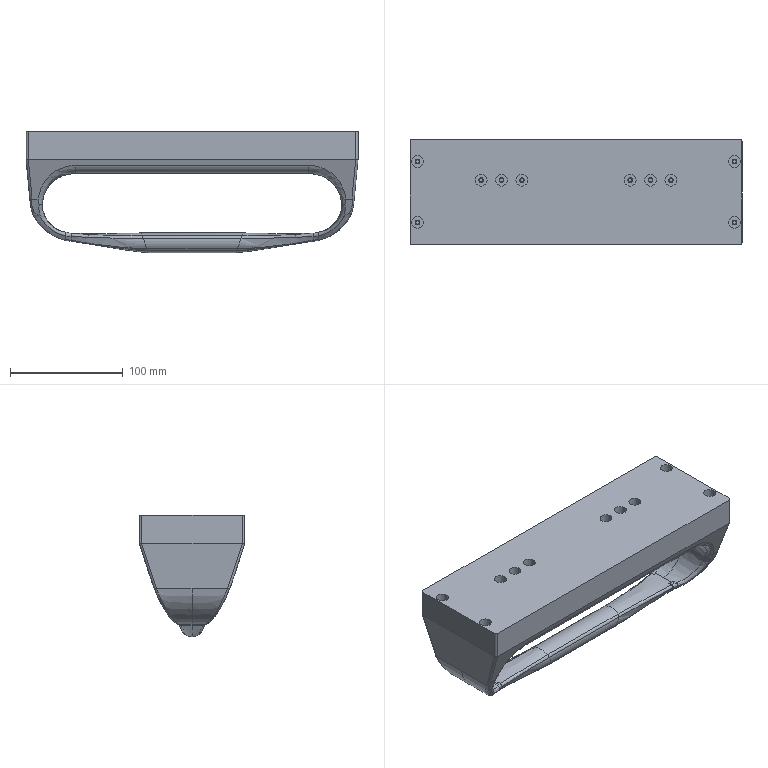NC program | NX | posted with a generic post | part box 294.078 x 93.5 x 107.5 mm
Lines 259 to 1268 of 185821:
(FIXED_CONTOUR , TOOL : D10R2)
N510 T09 M6
N512 G54
N514 G17 G0 G90 X46.702 Y-88.559 B0. C0. S7500 M3
N516 G43 Z30. H9
N518 Z-38.
N520 G94 G1 Z-40.107 F1000.
N522 X46.572 Y-88.43 Z-40.758
N524 X46.19 Y-88.155 Z-41.249
N526 X45.652 Y-87.879 Z-41.566
N528 X45.035 Y-87.652 Z-41.756
N530 X44.381 Y-87.48 Z-41.862
N532 X43.709 Y-87.358 Z-41.91
N534 X43.028 Y-87.278 Z-41.915
N536 X42.345 Y-87.233 Z-41.889
N538 X41.662 Y-87.22 Z-41.839
N540 X41.011 Z-41.785 F2500.
N542 X40.495 Z-41.758
N544 X39.805 Z-41.735
N546 X39.174 Z-41.73
N548 X20.152 Y-87.219
N550 X-39.177 Y-87.218 Z-41.726
N552 X-39.809 Z-41.732
N554 X-40.44 Z-41.755
N556 X-41.072 Z-41.793
N558 X-41.631 Z-41.84
N560 X-42.336 Y-87.186 Z-41.848
N562 X-42.568 Y-87.171 Z-41.851
N564 X-42.336 Z-41.821
N566 X-41.704 Z-41.756
N568 X-41.072 Z-41.705
N570 X-40.44 Z-41.669
N572 X-39.809 Z-41.648
N574 X-39.177 Z-41.642
N576 X17.515 Y-87.173 Z-41.646
N578 X32.819 Z-41.647
N580 X39.244 Z-41.646
N582 X39.805 Z-41.65
N584 X40.437 Z-41.67
N586 X41.069 Z-41.703
N588 X41.631 Z-41.748
N590 X41.701 Z-41.753
N592 X42.333 Z-41.817
N594 X42.596 Z-41.85
N596 X43.362 Y-87.127 Z-41.857
N598 X43.223 Z-41.836
N600 X42.965 Z-41.803
N602 X42.707 Z-41.775
N604 X42.333 Z-41.728
N606 X42.075 Z-41.704
N608 X41.701 Z-41.666
N610 X41.443 Z-41.651
N612 X41.069 Z-41.62
N614 X40.437 Z-41.587
N616 X40.179 Z-41.582
N618 X39.805 Z-41.57
N620 X39.174 Y-87.126 Z-41.566
N622 X15.94 Z-41.565
N624 X-39.177 Y-87.125 Z-41.562
N626 X-39.809 Z-41.567
N628 X-40.44 Z-41.587
N630 X-41.072 Z-41.622
N632 X-41.438 Z-41.652
N634 X-41.704 Z-41.669
N636 X-42.07 Z-41.708
N638 X-42.336 Z-41.732
N640 X-42.702 Z-41.78
N642 X-42.968 Z-41.809
N644 X-43.234 Z-41.844
N646 X-43.317 Z-41.857
N648 X-43.965 Y-87.079 Z-41.861
N650 X-43.416 Z-41.778
N652 X-42.968 Z-41.72
N654 X-42.52 Z-41.67
N656 X-42.336 Z-41.646
N658 X-41.888 Z-41.605
N660 X-41.704 Z-41.586
N662 X-41.256 Z-41.557
N664 X-41.072 Z-41.542
N666 X-40.44 Z-41.508
N668 X-39.809 Z-41.49
N670 X-39.177 Z-41.485
N672 X-20.221 Y-87.08 Z-41.486
N674 X39.174 Y-87.081 Z-41.488
N676 X39.805 Z-41.492
N678 X39.997 Z-41.498
N680 X40.437 Z-41.508
N682 X41.069 Z-41.54
N684 X41.261 Z-41.556
N686 X41.701 Z-41.582
N688 X41.893 Z-41.602
N690 X42.333 Z-41.642
N692 X42.522 Z-41.666
N694 X42.965 Z-41.714
N696 X43.405 Z-41.77
N698 X44.001 Z-41.86
N700 X44.599 Y-87.037 Z-41.863
N702 X43.581 Z-41.705
N704 X42.965 Z-41.627
N706 X42.333 Z-41.558
N708 X41.701 Z-41.501
N710 X41.069 Z-41.463
N712 X40.437 Z-41.43
N714 X39.805 Z-41.416
N716 X39.158 Z-41.413
N718 X-18.957 Y-87.036 Z-41.411
N720 X-33.494
N722 X-39.177 Z-41.41
N724 X-39.809 Y-87.035 Z-41.414
N726 X-40.44 Z-41.431
N728 X-41.08 Z-41.465
N730 X-41.704 Z-41.505
N732 X-42.343 Z-41.564
N734 X-42.97 Z-41.634
N736 X-43.593 Z-41.715
N738 X-44.228 Z-41.81
N740 X-44.561 Z-41.864
N742 X-45.125 Y-86.99 Z-41.867
N744 X-44.863 Z-41.82
N746 X-44.687 Z-41.795
N748 X-44.232 Z-41.721
N750 X-44.055 Z-41.698
N752 X-43.6 Z-41.63
N754 X-43.423 Z-41.611
N756 X-42.968 Z-41.552
N758 X-42.792 Z-41.535
N760 X-42.336 Z-41.484
N762 X-42.16 Z-41.47
N764 X-41.704 Z-41.428
N766 X-41.072 Z-41.389
N768 X-40.44 Z-41.357
N770 X-39.809 Z-41.342
N772 X-39.177 Z-41.338
N774 X-19.905 Z-41.339
N776 X39.342 Y-86.992 Z-41.341
N778 X39.805 Z-41.343
N780 X40.437 Z-41.356
N782 X41.237 Z-41.396
N784 X41.701 Z-41.424
N786 X42.165 Z-41.466
N788 X42.333 Z-41.479
N790 X42.796 Z-41.53
N792 X42.965 Z-41.545
N794 X43.428 Z-41.604
N796 X43.597 Z-41.622
N798 X43.765 Z-41.643
N800 X44.692 Z-41.787
N802 X45.028 Z-41.837
N804 X45.195 Z-41.867
N806 X45.492 Y-86.967 Z-41.868
N808 X45.707 Y-86.948 Z-41.867
N810 X45.206 Z-41.774
N812 X44.86 Z-41.721
N814 X44.514 Z-41.672
N816 X43.943 Y-86.947 Z-41.584
N818 X43.597 Z-41.54
N820 X43.25 Z-41.502
N822 X42.965 Z-41.466
N824 X42.618 Z-41.434
N826 X42.333 Z-41.403
N828 X41.986 Z-41.376
N830 X41.701 Z-41.35
N832 X41.069 Z-41.315
N834 X40.437 Z-41.284
N836 X39.805 Z-41.273
N838 X39.174 Z-41.271
N840 X-39.177 Y-86.946 Z-41.268
N842 X-39.809 Z-41.271
N844 X-40.086 Z-41.279
N846 X-40.44 Y-86.945 Z-41.285
N848 X-41.072 Z-41.316
N850 X-41.704 Z-41.354
N852 X-41.982 Z-41.379
N854 X-42.336 Z-41.407
N856 X-42.613 Z-41.439
N858 X-42.968 Z-41.473
N860 X-43.245 Z-41.509
N862 X-43.6 Z-41.547
N864 X-43.877 Z-41.589
N866 X-44.232 Z-41.634
N868 X-44.509 Z-41.68
N870 X-44.863 Z-41.73
N872 X-45.495 Z-41.843
N874 X-45.675 Z-41.87
N876 X-46.166 Y-86.902 Z-41.871
N878 X-45.759 Y-86.903 Z-41.794
N880 X-45.495 Z-41.755
N882 X-44.863 Z-41.643
N884 X-44.336 Z-41.568
N886 X-44.232 Z-41.551
N888 X-43.704 Z-41.483
N890 X-43.6 Z-41.467
N892 X-43.073 Z-41.41
N894 X-42.968 Z-41.396
N896 X-42.441 Z-41.345
N898 X-42.336 Z-41.334
N900 X-41.704 Z-41.282
N902 X-41.072 Z-41.245
N904 X-40.44 Z-41.216
N906 X-39.703 Z-41.203
N908 X-39.177 Z-41.2
N910 X39.174 Y-86.905 Z-41.203
N912 X39.805 Z-41.205
N914 X40.437 Z-41.215
N916 X41.069 Z-41.244
N918 X41.701 Z-41.278
N920 X42.333 Z-41.33
N922 X42.446 Z-41.342
N924 X42.965 Z-41.39
N926 X43.078 Z-41.404
N928 X43.597 Z-41.461
N930 X44.115 Z-41.526
N932 X44.341 Z-41.561
N934 X44.86 Z-41.634
N936 X45.379 Z-41.713
N938 X45.751 Z-41.783
N940 X46.175 Z-41.865
N942 X46.424 Y-86.884 Z-41.864
N944 X46.662 Y-86.862 Z-41.863
N946 X46.469 Z-41.823
N948 X46.124 Z-41.765
N950 X45.837 Z-41.708
N952 X45.55 Z-41.654
N954 X44.86 Z-41.55
N956 X44.228 Z-41.462
N958 X43.597 Z-41.384
N960 X43.023 Z-41.321
N962 X42.333 Z-41.259
N964 X41.701 Z-41.209
N966 X41.011 Z-41.175
N968 X40.437 Z-41.149
N970 X39.805 Z-41.139
N972 X37.59 Z-41.138
N974 X-39.177 Y-86.86 Z-41.135
N976 X-39.874 Z-41.139
N978 X-40.506 Z-41.152
N980 X-41.138 Z-41.181
N982 X-41.77 Z-41.217
N984 X-42.402 Z-41.268
N986 X-43.034 Z-41.328
N988 X-43.666 Z-41.397
N990 X-44.298 Z-41.478
N992 X-44.93 Z-41.567
N994 X-45.495 Z-41.668
N996 X-45.844 Z-41.719
N998 X-46.127 Z-41.773
N1000 X-46.476 Z-41.832
N1002 X-46.646 Z-41.867
N1004 X-46.87 Y-86.836 Z-41.858
N1006 X-46.985 Y-86.818 Z-41.839
N1008 X-46.759 Z-41.798
N1010 X-46.56 Z-41.757
N1012 X-46.127 Z-41.684
N1014 X-45.928 Z-41.645
N1016 X-45.495 Z-41.582
N1018 X-45.097 Z-41.512
N1020 X-44.465 Z-41.423
N1022 X-43.833 Z-41.342
N1024 X-43.201 Z-41.274
N1026 X-42.57 Z-41.215
N1028 X-41.938 Z-41.165
N1030 X-41.704 Z-41.149
N1032 X-41.306 Z-41.127
N1034 X-40.44 Z-41.089
N1036 X-39.809 Z-41.078
N1038 X-39.177 Y-86.819 Z-41.075
N1040 X39.399 Y-86.82 Z-41.077
N1042 X39.805 Z-41.078
N1044 X40.437 Z-41.089
N1046 X41.295 Z-41.125
N1048 X41.701 Z-41.146
N1050 X41.926 Z-41.161
N1052 X42.558 Z-41.21
N1054 X43.19 Z-41.268
N1056 X43.822 Z-41.336
N1058 X44.454 Z-41.414
N1060 X45.085 Y-86.821 Z-41.502
N1062 X45.492 Z-41.564
N1064 X45.717 Z-41.596
N1066 X46.124 Z-41.675
N1068 X46.552 Z-41.748
N1070 X46.756 Z-41.789
N1072 X47.067 Z-41.846
N1074 X47.236 Y-86.797 Z-41.826
N1076 X46.756 Z-41.738
N1078 X46.599 Z-41.706
N1080 X46.124 Z-41.625
N1082 X45.81 Z-41.564
N1084 X45.492 Z-41.519
N1086 X45.179 Z-41.471
N1088 X44.547 Z-41.383
N1090 X43.915 Z-41.305
N1092 X43.283 Z-41.238
N1094 X42.651 Z-41.18
N1096 X42.333 Z-41.157
N1098 X42.02 Z-41.132
N1100 X41.701 Z-41.111
N1102 X41.388 Z-41.094
N1104 X40.437 Z-41.055
N1106 X39.805 Z-41.044
N1108 X35.145 Z-41.043
N1110 X-39.177 Y-86.795 Z-41.041
N1112 X-39.809 Z-41.044
N1114 X-40.44 Z-41.055
N1116 X-40.767 Z-41.068
N1118 X-41.399 Z-41.097
N1120 X-41.704 Z-41.114
N1122 X-42.031 Z-41.136
N1124 X-42.663 Z-41.185
N1126 X-43.295 Z-41.244
N1128 X-43.927 Z-41.312
N1130 X-44.558 Z-41.392
N1132 X-45.19 Z-41.481
N1134 X-45.495 Z-41.535
N1136 X-45.975 Z-41.605
N1138 X-46.127 Z-41.634
N1140 X-46.607 Z-41.715
N1142 X-46.759 Z-41.747
N1144 X-47.132 Z-41.814
N1146 X-47.301 Y-86.768 Z-41.785
N1148 X-46.759 Z-41.687
N1150 X-46.661 Z-41.667
N1152 X-46.127 Z-41.576
N1154 X-46.029 Z-41.557
N1156 X-45.495 Z-41.479
N1158 X-45.299 Z-41.444
N1160 X-44.667 Z-41.356
N1162 X-44.035 Z-41.277
N1164 X-43.403 Z-41.209
N1166 X-42.771 Z-41.151
N1168 X-42.139 Z-41.102
N1170 X-41.704 Z-41.073
N1172 X-41.507 Z-41.062
N1174 X-40.875 Z-41.033
N1176 X-40.44 Z-41.016
N1178 X-39.809 Z-41.005
N1180 X-39.177 Z-41.002
N1182 X39.601 Y-86.77 Z-41.004
N1184 X39.805 Z-41.005
N1186 X40.437 Z-41.016
N1188 X41.496 Z-41.059
N1190 X41.701 Z-41.07
N1192 X42.128 Z-41.099
N1194 X42.76 Z-41.146
N1196 X43.391 Z-41.204
N1198 X44.023 Z-41.27
N1200 X44.655 Z-41.348
N1202 X45.287 Z-41.435
N1204 X45.492 Z-41.467
N1206 X45.919 Z-41.527
N1208 X46.124 Z-41.567
N1210 X46.653 Z-41.657
N1212 X46.756 Z-41.678
N1214 X47.285 Y-86.771 Z-41.774
N1216 X47.387 Z-41.798
N1218 X47.549 Y-86.744 Z-41.766
N1220 X47.388 Z-41.735
N1222 X47.339 Z-41.724
N1224 X46.707 Z-41.608
N1226 X46.076 Y-86.743 Z-41.499
N1228 X46.027 Z-41.49
N1230 X45.395 Z-41.399
N1232 X44.763 Z-41.312
N1234 X44.132 Z-41.235
N1236 X43.5 Z-41.169
N1238 X42.868 Z-41.111
N1240 X42.236 Z-41.065
N1242 X41.701 Z-41.029
N1244 X40.437 Z-40.977
N1246 X39.805 Z-40.965
N1248 X-39.177 Y-86.741 Z-40.963
N1250 X-39.809 Z-40.966
N1252 X-40.44 Z-40.977
N1254 X-40.984 Z-40.998
N1256 X-41.704 Z-41.032
N1258 X-42.336 Z-41.075
N1260 X-42.879 Z-41.117
N1262 X-43.511 Z-41.174
N1264 X-44.143 Z-41.242
N1266 X-44.775 Z-41.321
N1268 X-45.407 Z-41.408
N1270 X-45.495 Z-41.424
N1272 X-46.083 Z-41.51
N1274 X-46.715 Z-41.618
N1276 X-47.347 Z-41.733
N1278 X-47.464 Z-41.758
N1280 X-47.619 Y-86.715 Z-41.729
N1282 X-47.374 Z-41.681
N1284 X-46.759 Z-41.57
N1286 X-46.144 Z-41.466
N1288 X-45.495 Z-41.371
N1290 X-44.863 Z-41.285
N1292 X-44.248 Z-41.208
N1294 X-43.616 Z-41.141
N1296 X-42.984 Z-41.083
N1298 X-42.352 Z-41.035
N1300 X-41.704 Z-40.993
N1302 X-41.08 Z-40.964
N1304 X-40.449 Z-40.94
N1306 X-39.817 Z-40.929
N1308 X-39.177 Z-40.925
N1310 X39.805 Y-86.717 Z-40.927
N1312 X40.437 Z-40.939
N1314 X41.709 Z-40.99
N1316 X42.333 Z-41.032
N1318 X42.973 Z-41.078
N1320 X43.597 Z-41.135
N1322 X44.228 Z-41.2
N1324 X44.868 Z-41.278
N1326 X45.5 Z-41.364
N1328 X46.132 Z-41.454
N1330 X46.764 Z-41.561
N1332 X47.388 Z-41.675
N1334 X47.702 Z-41.735
N1336 X47.851 Y-86.69 Z-41.705
N1338 X47.388 Z-41.617
N1340 X46.874 Z-41.523
N1342 X46.242 Z-41.417
N1344 X45.61 Z-41.328
N1346 X45.492 Z-41.314
N1348 X44.978 Z-41.244
N1350 X44.228 Z-41.155
N1352 X43.597 Z-41.091
N1354 X43.083 Z-41.044
N1356 X42.333 Z-40.991
N1358 X41.819 Z-40.956
N1360 X40.496 Z-40.905
N1362 X39.805 Z-40.89
N1364 X-39.177 Y-86.688 Z-40.889
N1366 X-39.872 Z-40.894
N1368 X-40.504 Z-40.905
N1370 X-41.135 Z-40.929
N1372 X-41.83 Z-40.959
N1374 X-42.462 Z-41.001
N1376 X-43.094 Z-41.05
N1378 X-43.726 Z-41.108
N1380 X-44.358 Z-41.175
N1382 X-44.863 Z-41.238
N1384 X-44.99 Z-41.252
N1386 X-45.495 Z-41.322
N1388 X-45.622 Z-41.337
N1390 X-46.254 Z-41.429
N1392 X-46.759 Z-41.514
N1394 X-47.264 Z-41.606
N1396 X-47.391 Z-41.626
N1398 X-47.767 Z-41.701
N1400 X-47.923 Y-86.659 Z-41.671
N1402 X-47.391 Z-41.566
N1404 X-47.15 Z-41.527
N1406 X-46.759 Z-41.457
N1408 X-46.368 Z-41.39
N1410 X-45.736 Z-41.299
N1412 X-45.495 Z-41.27
N1414 X-45.104 Y-86.66 Z-41.216
N1416 X-44.863 Z-41.19
N1418 X-44.472 Z-41.141
N1420 X-43.841 Z-41.073
N1422 X-43.209 Z-41.014
N1424 X-42.577 Z-40.966
N1426 X-41.945 Z-40.924
N1428 X-41.704 Z-40.916
N1430 X-41.193 Z-40.893
N1432 X-40.44 Z-40.865
N1434 X-39.809 Z-40.855
N1436 X-39.177 Z-40.852
N1438 X39.174 Y-86.661 Z-40.853
N1440 X39.406 Z-40.851
N1442 X39.805 Y-86.662 Z-40.852
N1444 X40.437 Z-40.865
N1446 X41.185 Z-40.892
N1448 X41.934 Z-40.921
N1450 X42.565 Z-40.963
N1452 X43.197 Z-41.009
N1454 X43.829 Z-41.067
N1456 X44.461 Z-41.134
N1458 X44.86 Z-41.183
N1460 X45.093 Z-41.209
N1462 X45.492 Z-41.263
N1464 X45.724 Z-41.29
N1466 X46.356 Z-41.379
N1468 X46.756 Z-41.447
N1470 X46.988 Z-41.484
N1472 X47.388 Z-41.557
N1474 X48.002 Z-41.674
N1476 X48.159 Y-86.633 Z-41.64
N1478 X48.02 Z-41.618
N1480 X47.388 Z-41.497
N1482 X47.102 Z-41.444
N1484 X46.756 Z-41.39
N1486 X46.47 Z-41.341
N1488 X45.838 Z-41.252
N1490 X45.492 Z-41.213
N1492 X45.206 Z-41.173
N1494 X44.86 Z-41.135
N1496 X44.574 Z-41.1
N1498 X43.943 Z-41.033
N1500 X43.311 Z-40.974
N1502 X42.679 Z-40.927
N1504 X42.047 Z-40.886
N1506 X41.242 Z-40.855
N1508 X41.069 Z-40.85
N1510 X40.61 Z-40.833
N1512 X40.091 Z-40.819
N1514 X39.805 Z-40.813
N1516 X39.52
N1518 X39.174 Z-40.816
N1520 X-39.177 Y-86.631 Z-40.815
N1522 X-39.986 Z-40.82
N1524 X-40.44 Z-40.828
N1526 X-40.618 Z-40.833
N1528 X-41.249 Z-40.856
N1530 X-41.704 Z-40.877
N1532 X-42.058 Z-40.889
N1534 X-42.69 Z-40.93
N1536 X-43.322 Z-40.979
N1538 X-43.954 Z-41.039
N1540 X-44.586 Z-41.107
N1542 X-44.863 Z-41.142
N1544 X-45.218 Z-41.181
N1546 X-45.495 Z-41.219
N1548 X-45.85 Z-41.261
N1550 X-46.482 Z-41.352
N1552 X-46.759 Z-41.399
N1554 X-47.036 Z-41.449
N1556 X-47.391 Z-41.506
N1558 X-48.023 Z-41.63
N1560 X-48.083 Z-41.64
N1562 X-48.246 Y-86.603 Z-41.607
N1564 X-48.023 Z-41.57
N1566 X-47.391 Z-41.447
N1568 X-46.924 Z-41.372
N1570 X-46.594 Z-41.314
N1572 X-45.962 Z-41.224
N1574 X-45.495 Z-41.169
N1576 X-45.33 Z-41.146
N1578 X-44.863 Z-41.094
N1580 X-44.698 Z-41.074
N1582 X-44.066 Z-41.005
N1584 X-43.434 Z-40.945
N1586 X-42.802 Y-86.604 Z-40.896
N1588 X-42.17 Z-40.855
N1590 X-41.704 Z-40.838
N1592 X-41.305 Z-40.82
N1594 X-40.673 Z-40.797
N1596 X-40.44 Z-40.791
N1598 X-39.809 Z-40.781
N1600 X-39.177 Z-40.778
N1602 X39.174 Y-86.605 Z-40.78
N1604 X39.632 Z-40.775
N1606 X39.805 Z-40.776
N1608 X40.666 Z-40.797
N1610 X41.069 Z-40.813
N1612 X41.298 Z-40.819
N1614 X42.159 Y-86.606 Z-40.852
N1616 X42.965 Z-40.905
N1618 X43.423 Z-40.94
N1620 X44.054 Z-40.999
N1622 X44.686 Z-41.067
N1624 X44.86 Z-41.088
N1626 X45.318 Z-41.139
N1628 X45.492 Z-41.163
N1630 X45.95 Z-41.215
N1632 X46.582 Z-41.304
N1634 X46.756 Z-41.334
N1636 X47.213 Z-41.406
N1638 X48.02 Z-41.559
N1640 X48.248 Z-41.596
N1642 X48.308 Z-41.609
N1644 X48.46 Y-86.577 Z-41.579
N1646 X48.306 Z-41.544
N1648 X48.02 Z-41.498
N1650 X47.329 Z-41.366
N1652 X46.697 Z-41.266
N1654 X46.065 Z-41.176
N1656 X45.492 Z-41.111
N1658 X45.433 Z-41.103
N1660 X44.17 Z-40.963
N1662 X43.538 Z-40.905
N1664 X42.906 Z-40.856
N1666 X42.274 Z-40.817
N1668 X41.356 Z-40.782
N1670 X41.069 Z-40.774
N1672 X40.724 Z-40.761
N1674 X39.805 Z-40.737
N1676 X39.174 Z-40.742
N1678 X-39.177 Y-86.575 Z-40.74
N1680 X-39.809 Z-40.743
N1682 X-40.44 Z-40.753
N1684 X-40.731 Z-40.761
N1686 X-41.363 Z-40.783
N1688 X-41.704 Z-40.799
N1690 X-42.286 Z-40.819
N1692 X-42.968 Z-40.864
N1694 X-43.6 Z-40.914
N1696 X-44.232 Z-40.975
N1698 X-45.445 Z-41.11
N1700 X-46.127 Z-41.193
N1702 X-46.709 Z-41.276
N1704 X-47.391 Z-41.387
N1706 X-48.023 Z-41.509
N1708 X-48.314 Z-41.557
N1710 X-48.405 Z-41.577
N1712 X-48.569 Y-86.545 Z-41.547
N1714 X-48.373 Z-41.504
N1716 X-48.023 Z-41.446
N1718 X-47.459 Z-41.337
N1720 X-47.322 Z-41.318
N1722 X-46.759 Z-41.227
N1724 X-46.127 Z-41.139
N1726 X-45.495 Z-41.066
N1728 X-44.932 Z-41.003
N1730 X-44.863 Z-40.997
N1732 X-44.3 Z-40.935
N1734 X-44.163 Z-40.924
N1736 X-43.6 Z-40.87
N1738 X-42.968 Z-40.821
N1740 X-42.268 Z-40.778
N1742 X-41.704 Z-40.758
N1744 X-41.422 Z-40.745
N1746 X-40.79 Z-40.723
N1748 X-40.44 Z-40.714
N1750 X-39.809 Z-40.704
N1752 X-39.177 Z-40.702
N1754 X39.174 Y-86.547 Z-40.704
N1756 X39.805 Z-40.698
N1758 X40.783 Z-40.723
N1760 X41.069 Z-40.734
N1762 X41.415 Z-40.744
N1764 X42.333 Z-40.779
N1766 X42.965 Z-40.817
N1768 X43.597 Z-40.866
N1770 X44.228 Z-40.923
N1772 X44.288 Z-40.928
N1774 X45.492 Z-41.06
N1776 X46.184 Z-41.138
N1778 X46.756 Y-86.548 Z-41.219
N1780 X47.388 Z-41.317
N1782 X47.447 Z-41.326
N1784 X48.02 Z-41.436
N1786 X48.365 Z-41.492
N1788 X48.62 Z-41.549
N1790 X48.799 Y-86.52 Z-41.522
N1792 X48.651 Z-41.495
N1794 X48.42 Z-41.443
N1796 X48.02 Z-41.378
N1798 X47.557 Z-41.289
N1800 X47.219 Z-41.241
N1802 X46.756 Z-41.169
N1804 X46.293 Z-41.103
N1806 X46.124 Z-41.083
N1808 X45.955 Z-41.067
N1810 X45.029 Z-40.963
N1812 X44.86 Z-40.948
N1814 X44.398 Z-40.897
N1816 X44.059 Z-40.87
N1818 X43.597 Z-40.827
N1820 X43.427 Z-40.816
N1822 X42.965 Z-40.78
N1824 X42.333 Z-40.743
N1826 X42.163 Z-40.735
N1828 X41.47 Z-40.709
N1830 X41.069 Z-40.698
N1832 X40.838 Z-40.689
N1834 X39.805 Z-40.663
N1836 X39.174 Z-40.668
N1838 X-39.177 Y-86.518 Z-40.666
N1840 X-39.809 Z-40.668
N1842 X-40.44 Z-40.678
N1844 X-40.845 Z-40.689
N1846 X-41.477 Z-40.71
N1848 X-41.704 Z-40.721
N1850 X-42.159 Z-40.737
N1852 X-42.336 Z-40.745
N1854 X-42.968 Z-40.784
N1856 X-43.422 Z-40.819
N1858 X-43.6 Z-40.831
N1860 X-44.054 Z-40.875
N1862 X-44.409 Z-40.903
N1864 X-44.863 Z-40.954
N1866 X-45.041 Z-40.969
N1868 X-45.495 Z-41.019
N1870 X-45.673 Z-41.037
N1872 X-46.305 Z-41.112
N1874 X-46.759 Z-41.177
N1876 X-47.213 Z-41.25
N1878 X-47.569 Z-41.3
N1880 X-48.023 Z-41.388
N1882 X-48.428 Z-41.455
N1884 X-48.655 Z-41.504
N1886 X-48.74 Z-41.52
N1888 X-48.914 Y-86.492 Z-41.494
N1890 X-48.655 Z-41.445
N1892 X-48.481 Z-41.408
N1894 X-48.023 Z-41.331
N1896 X-47.675 Z-41.264
N1898 X-47.107 Z-41.184
N1900 X-46.759 Z-41.128
N1902 X-46.411 Z-41.078
N1904 X-45.779 Z-41.002
N1906 X-45.495 Z-40.975
N1908 X-45.147 Z-40.936
N1910 X-44.863 Z-40.911
N1912 X-44.515 Z-40.873
N1914 X-43.948 Z-40.827
N1916 X-43.6 Z-40.793
N1918 X-43.316 Z-40.775
N1920 X-42.968 Z-40.748
N1922 X-42.685 Z-40.732
N1924 X-42.336 Z-40.71
N1926 X-42.053 Z-40.697
N1928 X-41.53 Z-40.676
N1930 X-40.898 Z-40.655
N1932 X-40.44 Z-40.643
N1934 X-39.809 Z-40.633
N1936 X-39.177 Z-40.631
N1938 X39.174 Y-86.494 Z-40.633
N1940 X39.805 Z-40.629
N1942 X40.081 Z-40.634
N1944 X40.891 Z-40.655
N1946 X41.069 Z-40.662
N1948 X41.523 Z-40.675
N1950 X42.057 Z-40.695
N1952 X42.333 Z-40.708
N1954 X42.689 Z-40.73
N1956 X42.965 Z-40.744
N1958 X43.321 Z-40.772
N1960 X43.597 Z-40.79
N1962 X43.953 Z-40.823
N1964 X44.228 Z-40.843
N1966 X44.503 Z-40.867
N1968 X44.86 Z-40.906
N1970 X45.135 Z-40.93
N1972 X45.849 Z-41.01
N1974 X46.124 Z-41.036
N1976 X46.399 Z-41.069
N1978 X46.756 Z-41.12
N1980 X47.113 Z-41.176
N1982 X47.662 Z-41.254
N1984 X48.016 Z-41.321
N1986 X48.473 Z-41.396
N1988 X48.651 Z-41.436
N1990 X48.975 Z-41.495
N1992 X49.147 Y-86.468 Z-41.469
N1994 X48.651 Z-41.378
N1996 X48.525 Z-41.349
N1998 X48.017 Z-41.267
N2000 X47.767 Z-41.219
N2002 X47.009 Z-41.112
N2004 X46.756 Z-41.072
N2006 X46.503 Z-41.036
N2008 X46.124 Z-40.99
N2010 X45.745 Z-40.954
N2012 X45.239 Z-40.898
N2014 X44.86 Z-40.865
N2016 X44.608 Z-40.837
N2018 X44.228 Z-40.805
N2020 X43.849 Z-40.777
N2022 X43.597 Z-40.753
N2024 X43.217 Z-40.728
N2026 X42.965 Z-40.709
N2028 X42.585 Z-40.689
N2030 X42.333 Z-40.674
N2032 X41.953 Z-40.656
N2034 X41.575 Z-40.641
N2036 X40.437 Z-40.609
N2038 X39.933 Z-40.598
N2040 X39.678 Z-40.596
N2042 X39.174 Z-40.599
N2044 X-39.299 Y-86.466 Z-40.598
N2046 X-39.809 Z-40.599
N2048 X-40.44 Z-40.608
N2050 X-41.072 Z-40.627
N2052 X-41.582 Z-40.643
N2054 X-41.948 Z-40.657
N2056 X-42.336 Z-40.675
N2058 X-42.58 Z-40.691
N2060 X-42.968 Z-40.712
N2062 X-43.212 Z-40.731
N2064 X-43.6 Z-40.756
N2066 X-43.844 Z-40.78
N2068 X-44.232 Z-40.81
N2070 X-44.619 Z-40.843
N2072 X-44.863 Z-40.87
N2074 X-45.251 Z-40.903
N2076 X-45.495 Z-40.931
N2078 X-45.883 Z-40.969
N2080 X-46.515 Z-41.045
N2082 X-46.759 Z-41.079
N2084 X-47.003 Z-41.119
N2086 X-47.779 Z-41.229
N2088 X-48.023 Z-41.276
N2090 X-48.533 Z-41.361
N2092 X-48.655 Z-41.387
N2094 X-49.086 Z-41.468
N2096 X-49.256 Y-86.439 Z-41.442
N2098 X-49.218 Z-41.433
N2100 X-48.655 Z-41.328
N2102 X-48.586 Z-41.313
N2104 X-48.023 Z-41.22
N2106 X-47.885 Z-41.193
N2108 X-46.897 Z-41.053
N2110 X-46.759 Z-41.03
N2112 X-46.621 Z-41.011
N2114 X-45.989 Z-40.934
N2116 X-45.495 Z-40.886
N2118 X-45.357 Y-86.44 Z-40.87
N2120 X-44.863 Z-40.827
N2122 X-44.725 Z-40.812
N2124 X-44.232 Z-40.77
N2126 X-43.738 Z-40.732
N2128 X-43.6 Z-40.719
N2130 X-43.106 Z-40.687
N2132 X-42.968 Z-40.676
N2134 X-42.336 Z-40.64
N2136 X-41.842 Z-40.617
N2138 X-41.003 Z-40.589
N2140 X-40.371 Z-40.572
N2142 X-39.809 Z-40.564
N2144 X-39.177 Z-40.562
N2146 X39.174 Y-86.441 Z-40.565
N2148 X39.805 Y-86.442 Z-40.563
N2150 X40.291 Z-40.57
N2152 X41.628 Z-40.607
N2154 X41.847 Z-40.615
N2156 X42.333 Z-40.639
N2158 X42.965 Z-40.673
N2160 X43.111 Z-40.684
N2162 X43.597 Z-40.716
N2164 X43.743 Z-40.73
N2166 X44.228 Z-40.765
N2168 X44.714 Z-40.807
N2170 X44.86 Z-40.823
N2172 X45.346 Z-40.865
N2174 X45.639 Z-40.898
N2176 X46.124 Z-40.944
N2178 X46.609 Z-41.002
N2180 X46.902 Z-41.046
N2182 X47.388 Z-41.113
N2184 X47.873 Z-41.183
N2186 X48.018 Z-41.211
N2188 X48.578 Z-41.302
N2190 X48.651 Z-41.318
N2192 X49.21 Z-41.421
N2194 X49.314 Z-41.444
N2196 X49.486 Y-86.415 Z-41.419
N2198 X49.262 Z-41.37
N2200 X48.632 Z-41.254
N2202 X47.98 Z-41.147
N2204 X47.388 Z-41.062
N2206 X46.717 Z-40.968
N2208 X46.124 Z-40.897
N2210 X45.453 Z-40.832
N2212 X44.228 Z-40.725
N2214 X43.597 Z-40.678
N2216 X42.965 Z-40.636
N2218 X41.74 Z-40.575
N2220 X40.36 Z-40.537
N2222 X39.805 Z-40.529
N2224 X-39.192 Y-86.413 Z-40.527
N2226 X-39.809 Z-40.529
N2228 X-40.44 Z-40.538
N2230 X-41.704 Z-40.575
N2232 X-42.367 Z-40.607
N2234 X-42.998 Z-40.642
N2236 X-43.63 Z-40.684
N2238 X-44.232 Z-40.73
N2240 X-45.495 Z-40.84
N2242 X-46.127 Z-40.903
N2244 X-46.759 Z-40.981
N2246 X-47.993 Z-41.157
N2248 X-48.655 Z-41.268
N2250 X-49.286 Z-41.387
N2252 X-49.426 Z-41.417
N2254 X-49.598 Y-86.385 Z-41.391
N2256 X-49.366 Z-41.342
N2258 X-48.734 Z-41.224
N2260 X-48.102 Z-41.119
N2262 X-47.471 Z-41.029
N2264 X-47.391 Z-41.021
N2266 X-46.799 Z-40.939
N2268 X-46.127 Z-40.858
N2270 X-45.495 Z-40.797
N2272 X-44.232 Z-40.69
N2274 X-43.6 Z-40.642
N2276 X-42.968 Y-86.386 Z-40.603
N2278 X-42.336 Z-40.569
N2280 X-41.783 Z-40.543
N2282 X-40.44 Z-40.505
N2284 X-39.809 Z-40.496
N2286 X-36.837 Z-40.495
N2288 X39.841 Y-86.387 Z-40.497
N2290 X40.473 Z-40.506
N2292 X41.772 Y-86.388 Z-40.541
N2294 X42.965 Z-40.6
N2296 X43.597 Z-40.64
N2298 X44.299 Z-40.691
N2300 X45.492 Z-40.793
N2302 X46.195 Z-40.86
N2304 X46.827 Z-40.935
N2306 X47.388 Z-41.012
N2308 X47.458 Z-41.02
N2310 X48.09 Z-41.11
N2312 X48.651 Z-41.201
N2314 X49.213 Z-41.304
N2316 X49.354 Z-41.328
N2318 X49.66 Z-41.393
N2320 X49.839 Y-86.359 Z-41.367
N2322 X49.468 Z-41.288
N2324 X49.283 Z-41.255
N2326 X49.098 Z-41.226
N2328 X48.651 Z-41.144
N2330 X48.204 Z-41.072
N2332 X48.02 Z-41.048
N2334 X47.573 Z-40.984
N2336 X47.388 Z-40.964
N2338 X46.941 Z-40.902
N2340 X46.756 Z-40.882
N2342 X46.309 Z-40.828
N2344 X46.124 Z-40.808
N2346 X45.939 Z-40.792
N2348 X45.492 Z-40.75
N2350 X44.414 Z-40.658
N2352 X44.043 Z-40.634
N2354 X43.597 Z-40.601
N2356 X43.411 Z-40.591
N2358 X42.965 Z-40.562
N2360 X42.779 Z-40.554
N2362 X41.886 Z-40.509
N2364 X40.437 Z-40.473
N2366 X39.805 Z-40.464
N2368 X-39.273 Y-86.357 Z-40.462
N2370 X-39.905 Z-40.464
N2372 X-40.537 Z-40.474
N2374 X-41.169 Z-40.49
N2376 X-41.898 Z-40.511
N2378 X-42.336 Z-40.532
N2380 X-42.774 Z-40.556
N2382 X-42.968 Z-40.564
N2384 X-43.406 Z-40.593
N2386 X-43.6 Z-40.603
N2388 X-44.038 Z-40.637
N2390 X-44.425 Z-40.663
N2392 X-45.495 Z-40.754
N2394 X-45.933 Z-40.797
N2396 X-46.127 Z-40.814
N2398 X-46.321 Z-40.835
N2400 X-46.759 Z-40.889
N2402 X-46.953 Z-40.91
N2404 X-47.391 Z-40.971
N2406 X-47.585 Z-40.992
N2408 X-48.023 Z-41.056
N2410 X-48.217 Z-41.081
N2412 X-48.849 Z-41.184
N2414 X-49.481 Z-41.301
N2416 X-49.774 Z-41.365
N2418 X-49.963 Y-86.327 Z-41.337
N2420 X-49.6 Z-41.26
N2422 X-48.968 Z-41.143
N2424 X-48.655 Z-41.094
N2426 X-48.336 Z-41.041
N2428 X-48.023 Z-41.
N2430 X-47.704 Z-40.954
N2432 X-47.391 Z-40.919
N2434 X-47.072 Z-40.875
N2436 X-46.916 Z-40.856
N2438 X-46.759 Z-40.841
N2440 X-46.44 Z-40.802
N2442 X-46.127 Z-40.767
N2444 X-45.814 Z-40.741
N2446 X-45.495 Z-40.709
N2448 X-44.544 Z-40.629
N2450 X-44.232 Z-40.606
N2452 X-43.919 Z-40.586
N2454 X-43.6 Z-40.562
N2456 X-43.287 Z-40.545
N2458 X-42.968 Z-40.525
N2460 X-42.655 Z-40.511
N2462 X-42.017 Z-40.479
N2464 X-41.704 Z-40.471
N2466 X-41.229 Y-86.328 Z-40.457
N2468 X-40.44 Z-40.437
N2470 X-39.809 Z-40.429
N2472 X39.805 Y-86.329 Z-40.43
N2474 X40.59 Z-40.441
N2476 X42.006 Z-40.477
N2478 X42.66 Z-40.51
N2480 X42.965 Z-40.522
N2482 X43.292 Y-86.33 Z-40.544
N2484 X43.597 Z-40.56
N2486 X43.924 Z-40.584
N2488 X44.228 Z-40.603
N2490 X44.533 Z-40.625
N2492 X45.492 Z-40.705
N2494 X45.82 Z-40.736
N2496 X46.124 Z-40.761
N2498 X46.428 Z-40.794
N2500 X46.756 Z-40.834
N2502 X46.908 Z-40.849
N2504 X47.06 Z-40.867
N2506 X47.388 Z-40.912
N2508 X47.692 Z-40.946
N2510 X48.02 Z-40.993
N2512 X48.324 Z-41.032
N2514 X48.651 Z-41.085
N2516 X48.979 Z-41.145
N2518 X49.283 Z-41.192
N2520 X49.587 Z-41.246
N2522 X49.915 Z-41.317